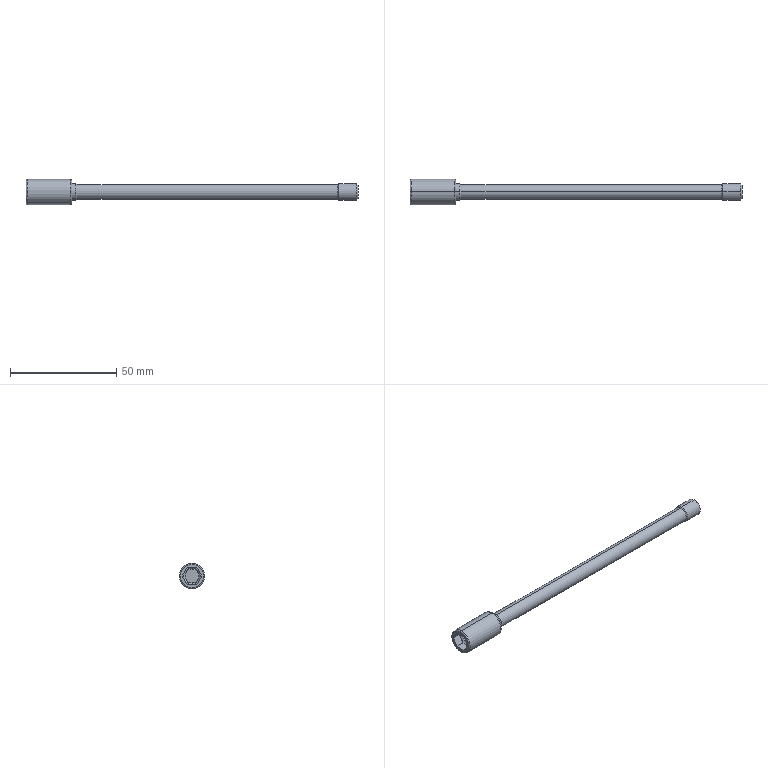Part | STEP file | SC63_752 | 1 solid | 40 faces | box 156.5 x 12 x 12 mm | volume 7243 mm3 | plane 16 | cone 10 | cylinder 10 | torus 4 | commonest cylinder face diameters 8 x4 6.647 x2 7.06 x2 12 x2